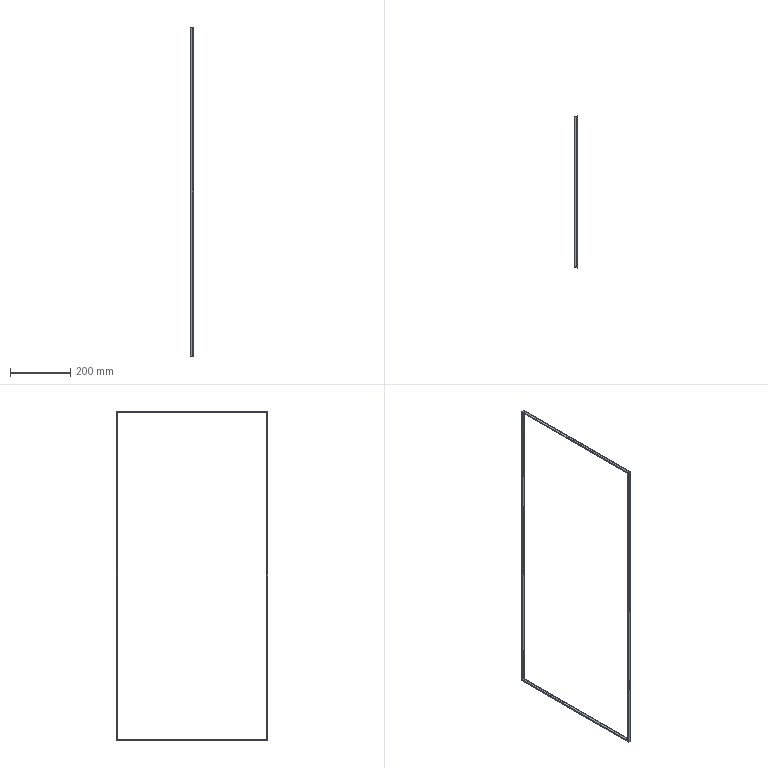Part | STEP file | RJWD-DY-0102_X2_5DE667DC95E8_22 | 1 solid | 36 faces | box 10 x 501.011 x 1091 mm | volume 114606 mm3 | plane 20 | cylinder 16 | commonest cylinder face diameters 2 x16